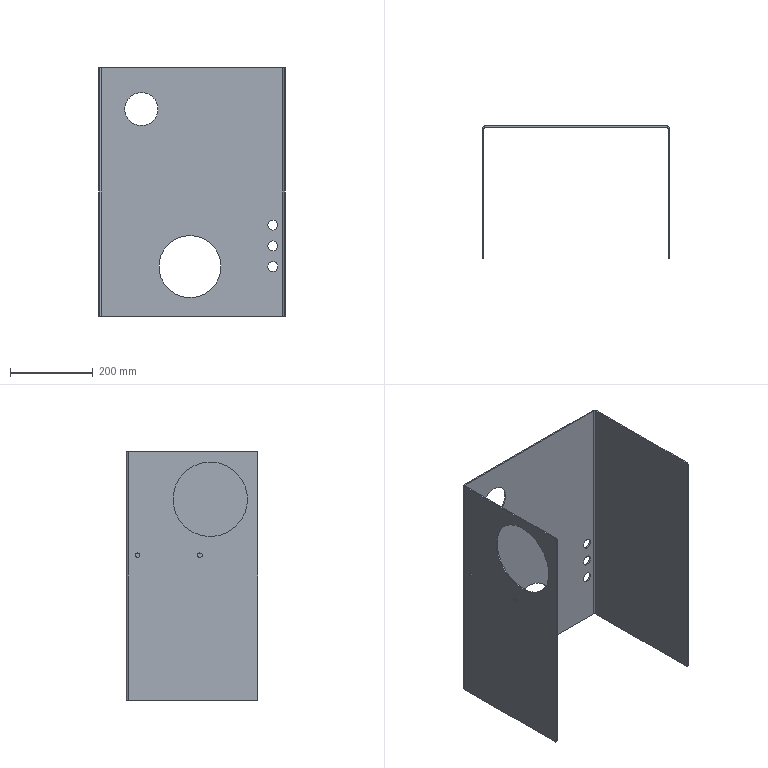Part | SolidWorks | features ICE 3, FlatPattern 1, SMBaseFlange 1, SheetMetal 1 | 1 solid | 42 faces | box 450 x 318 x 600 mm | volume 1787947 mm3 | cylinder 24 | plane 18 | commonest cylinder face diameters 6 x6 24 x6 11 x4 12 x2 80 x2 150 x2
STEP:
#1=CARTESIAN_POINT('',(3.,140.,344.5));
#2=VERTEX_POINT('',#1);
#3=CARTESIAN_POINT('',(3.,140.,355.5));
#4=VERTEX_POINT('',#3);
#5=CARTESIAN_POINT('',(3.,140.,350.));
#6=DIRECTION('',(-1.,0.,0.));
#7=DIRECTION('',(0.,0.,1.));
#8=AXIS2_PLACEMENT_3D('',#5,#6,#7);
#9=CIRCLE('',#8,5.5);
#10=EDGE_CURVE('',#2,#4,#9,.T.);
#11=ORIENTED_EDGE('',*,*,#10,.F.);
#12=CARTESIAN_POINT('',(0.,140.,344.5));
#13=VERTEX_POINT('',#12);
#14=CARTESIAN_POINT('',(10.,140.,344.5));
#15=DIRECTION('',(-1.,0.,0.));
#16=VECTOR('',#15,1000.);
#17=LINE('',#14,#16);
#18=EDGE_CURVE('',#2,#13,#17,.T.);
#19=ORIENTED_EDGE('',*,*,#18,.T.);
#20=CARTESIAN_POINT('',(0.,140.,355.5));
#21=VERTEX_POINT('',#20);
#22=CARTESIAN_POINT('',(0.,140.,350.));
#23=DIRECTION('',(-1.,0.,0.));
#24=DIRECTION('',(0.,0.,1.));
#25=AXIS2_PLACEMENT_3D('',#22,#23,#24);
#26=CIRCLE('',#25,5.5);
#27=EDGE_CURVE('',#13,#21,#26,.T.);
#28=ORIENTED_EDGE('',*,*,#27,.T.);
#29=CARTESIAN_POINT('',(10.,140.,355.5));
#30=DIRECTION('',(-1.,0.,0.));
#31=VECTOR('',#30,1000.);
#32=LINE('',#29,#31);
#33=EDGE_CURVE('',#4,#21,#32,.T.);
#34=ORIENTED_EDGE('',*,*,#33,.F.);
#35=EDGE_LOOP('',(#11,#19,#28,#34));
#36=FACE_OUTER_BOUND('',#35,.T.);
#37=CARTESIAN_POINT('',(10.,140.,350.));
#38=DIRECTION('',(-1.,0.,0.));
#39=DIRECTION('',(0.,0.,1.));
#40=AXIS2_PLACEMENT_3D('',#37,#38,#39);
#41=CYLINDRICAL_SURFACE('',#40,5.5);
#42=ADVANCED_FACE('',(#36),#41,.F.);
#43=CARTESIAN_POINT('',(3.,290.,344.5));
#44=VERTEX_POINT('',#43);
#45=CARTESIAN_POINT('',(3.,290.,355.5));
#46=VERTEX_POINT('',#45);
#47=CARTESIAN_POINT('',(3.,290.,350.));
#48=DIRECTION('',(-1.,0.,0.));
#49=DIRECTION('',(0.,0.,1.));
#50=AXIS2_PLACEMENT_3D('',#47,#48,#49);
#51=CIRCLE('',#50,5.5);
#52=EDGE_CURVE('',#44,#46,#51,.T.);
#53=ORIENTED_EDGE('',*,*,#52,.F.);
#54=CARTESIAN_POINT('',(0.,290.,344.5));
#55=VERTEX_POINT('',#54);
#56=CARTESIAN_POINT('',(10.,290.,344.5));
#57=DIRECTION('',(-1.,0.,0.));
#58=VECTOR('',#57,1000.);
#59=LINE('',#56,#58);
#60=EDGE_CURVE('',#44,#55,#59,.T.);
#61=ORIENTED_EDGE('',*,*,#60,.T.);
#62=CARTESIAN_POINT('',(0.,290.,355.5));
#63=VERTEX_POINT('',#62);
#64=CARTESIAN_POINT('',(0.,290.,350.));
#65=DIRECTION('',(-1.,0.,0.));
#66=DIRECTION('',(0.,0.,1.));
#67=AXIS2_PLACEMENT_3D('',#64,#65,#66);
#68=CIRCLE('',#67,5.5);
#69=EDGE_CURVE('',#55,#63,#68,.T.);
#70=ORIENTED_EDGE('',*,*,#69,.T.);
#71=CARTESIAN_POINT('',(10.,290.,355.5));
#72=DIRECTION('',(-1.,0.,0.));
#73=VECTOR('',#72,1000.);
#74=LINE('',#71,#73);
#75=EDGE_CURVE('',#46,#63,#74,.T.);
#76=ORIENTED_EDGE('',*,*,#75,.F.);
#77=EDGE_LOOP('',(#53,#61,#70,#76));
#78=FACE_OUTER_BOUND('',#77,.T.);
#79=CARTESIAN_POINT('',(10.,290.,350.));
#80=DIRECTION('',(-1.,0.,0.));
#81=DIRECTION('',(0.,0.,1.));
#82=AXIS2_PLACEMENT_3D('',#79,#80,#81);
#83=CYLINDRICAL_SURFACE('',#82,5.5);
#84=ADVANCED_FACE('',(#78),#83,.F.);
#85=CARTESIAN_POINT('',(3.,115.,395.));
#86=VERTEX_POINT('',#85);
#87=CARTESIAN_POINT('',(3.,115.,575.));
#88=VERTEX_POINT('',#87);
#89=CARTESIAN_POINT('',(3.,115.,485.));
#90=DIRECTION('',(-1.,0.,0.));
#91=DIRECTION('',(0.,0.,1.));
#92=AXIS2_PLACEMENT_3D('',#89,#90,#91);
#93=CIRCLE('',#92,90.);
#94=EDGE_CURVE('',#86,#88,#93,.T.);
#95=ORIENTED_EDGE('',*,*,#94,.F.);
#96=CARTESIAN_POINT('',(0.,115.,395.));
#97=VERTEX_POINT('',#96);
#98=CARTESIAN_POINT('',(10.,115.,395.));
#99=DIRECTION('',(-1.,0.,0.));
#100=VECTOR('',#99,1000.);
#101=LINE('',#98,#100);
#102=EDGE_CURVE('',#86,#97,#101,.T.);
#103=ORIENTED_EDGE('',*,*,#102,.T.);
#104=CARTESIAN_POINT('',(0.,115.,575.));
#105=VERTEX_POINT('',#104);
#106=CARTESIAN_POINT('',(0.,115.,485.));
#107=DIRECTION('',(-1.,0.,0.));
#108=DIRECTION('',(0.,0.,1.));
#109=AXIS2_PLACEMENT_3D('',#106,#107,#108);
#110=CIRCLE('',#109,90.);
#111=EDGE_CURVE('',#97,#105,#110,.T.);
#112=ORIENTED_EDGE('',*,*,#111,.T.);
#113=CARTESIAN_POINT('',(10.,115.,575.));
#114=DIRECTION('',(-1.,0.,0.));
#115=VECTOR('',#114,1000.);
#116=LINE('',#113,#115);
#117=EDGE_CURVE('',#88,#105,#116,.T.);
#118=ORIENTED_EDGE('',*,*,#117,.F.);
#119=EDGE_LOOP('',(#95,#103,#112,#118));
#120=FACE_OUTER_BOUND('',#119,.T.);
#121=CARTESIAN_POINT('',(10.,115.,485.));
#122=DIRECTION('',(-1.,0.,0.));
#123=DIRECTION('',(0.,0.,1.));
#124=AXIS2_PLACEMENT_3D('',#121,#122,#123);
#125=CYLINDRICAL_SURFACE('',#124,90.);
#126=ADVANCED_FACE('',(#120),#125,.F.);
#127=CARTESIAN_POINT('',(103.,315.,460.));
#128=VERTEX_POINT('',#127);
#129=CARTESIAN_POINT('',(103.,315.,540.));
#130=VERTEX_POINT('',#129);
#131=CARTESIAN_POINT('',(103.,315.,500.));
#132=DIRECTION('',(0.,1.,0.));
#133=DIRECTION('',(0.,0.,1.));
#134=AXIS2_PLACEMENT_3D('',#131,#132,#133);
#135=CIRCLE('',#134,40.);
#136=EDGE_CURVE('',#128,#130,#135,.T.);
#137=ORIENTED_EDGE('',*,*,#136,.F.);
#138=CARTESIAN_POINT('',(103.,318.,460.));
#139=VERTEX_POINT('',#138);
#140=CARTESIAN_POINT('',(103.,308.,460.));
#141=DIRECTION('',(0.,1.,0.));
#142=VECTOR('',#141,1000.);
#143=LINE('',#140,#142);
#144=EDGE_CURVE('',#128,#139,#143,.T.);
#145=ORIENTED_EDGE('',*,*,#144,.T.);
#146=CARTESIAN_POINT('',(103.,318.,540.));
#147=VERTEX_POINT('',#146);
#148=CARTESIAN_POINT('',(103.,318.,500.));
#149=DIRECTION('',(0.,1.,0.));
#150=DIRECTION('',(0.,0.,1.));
#151=AXIS2_PLACEMENT_3D('',#148,#149,#150);
#152=CIRCLE('',#151,40.);
#153=EDGE_CURVE('',#139,#147,#152,.T.);
#154=ORIENTED_EDGE('',*,*,#153,.T.);
#155=CARTESIAN_POINT('',(103.,308.,540.));
#156=DIRECTION('',(0.,1.,0.));
#157=VECTOR('',#156,1000.);
#158=LINE('',#155,#157);
#159=EDGE_CURVE('',#130,#147,#158,.T.);
#160=ORIENTED_EDGE('',*,*,#159,.F.);
#161=EDGE_LOOP('',(#137,#145,#154,#160));
#162=FACE_OUTER_BOUND('',#161,.T.);
#163=CARTESIAN_POINT('',(103.,308.,500.));
#164=DIRECTION('',(0.,1.,0.));
#165=DIRECTION('',(0.,0.,1.));
#166=AXIS2_PLACEMENT_3D('',#163,#164,#165);
#167=CYLINDRICAL_SURFACE('',#166,40.);
#168=ADVANCED_FACE('',(#162),#167,.F.);
#169=CARTESIAN_POINT('',(220.,315.,45.));
#170=VERTEX_POINT('',#169);
#171=CARTESIAN_POINT('',(220.,315.,195.));
#172=VERTEX_POINT('',#171);
#173=CARTESIAN_POINT('',(220.,315.,120.));
#174=DIRECTION('',(0.,1.,0.));
#175=DIRECTION('',(0.,0.,1.));
#176=AXIS2_PLACEMENT_3D('',#173,#174,#175);
#177=CIRCLE('',#176,75.);
#178=EDGE_CURVE('',#170,#172,#177,.T.);
#179=ORIENTED_EDGE('',*,*,#178,.F.);
#180=CARTESIAN_POINT('',(220.,318.,45.));
#181=VERTEX_POINT('',#180);
#182=CARTESIAN_POINT('',(220.,308.,45.));
#183=DIRECTION('',(0.,1.,0.));
#184=VECTOR('',#183,1000.);
#185=LINE('',#182,#184);
#186=EDGE_CURVE('',#170,#181,#185,.T.);
#187=ORIENTED_EDGE('',*,*,#186,.T.);
#188=CARTESIAN_POINT('',(220.,318.,195.));
#189=VERTEX_POINT('',#188);
#190=CARTESIAN_POINT('',(220.,318.,120.));
#191=DIRECTION('',(0.,1.,0.));
#192=DIRECTION('',(0.,0.,1.));
#193=AXIS2_PLACEMENT_3D('',#190,#191,#192);
#194=CIRCLE('',#193,75.);
#195=EDGE_CURVE('',#181,#189,#194,.T.);
#196=ORIENTED_EDGE('',*,*,#195,.T.);
#197=CARTESIAN_POINT('',(220.,308.,195.));
#198=DIRECTION('',(0.,1.,0.));
#199=VECTOR('',#198,1000.);
#200=LINE('',#197,#199);
#201=EDGE_CURVE('',#172,#189,#200,.T.);
#202=ORIENTED_EDGE('',*,*,#201,.F.);
#203=EDGE_LOOP('',(#179,#187,#196,#202));
#204=FACE_OUTER_BOUND('',#203,.T.);
#205=CARTESIAN_POINT('',(220.,308.,120.));
#206=DIRECTION('',(0.,1.,0.));
#207=DIRECTION('',(0.,0.,1.));
#208=AXIS2_PLACEMENT_3D('',#205,#206,#207);
#209=CYLINDRICAL_SURFACE('',#208,75.);
#210=ADVANCED_FACE('',(#204),#209,.F.);
#211=CARTESIAN_POINT('',(420.,315.,208.));
#212=VERTEX_POINT('',#211);
#213=CARTESIAN_POINT('',(420.,315.,232.));
#214=VERTEX_POINT('',#213);
#215=CARTESIAN_POINT('',(420.,315.,220.));
#216=DIRECTION('',(0.,1.,0.));
#217=DIRECTION('',(0.,0.,1.));
#218=AXIS2_PLACEMENT_3D('',#215,#216,#217);
#219=CIRCLE('',#218,12.);
#220=EDGE_CURVE('',#212,#214,#219,.T.);
#221=ORIENTED_EDGE('',*,*,#220,.F.);
#222=CARTESIAN_POINT('',(420.,318.,208.));
#223=VERTEX_POINT('',#222);
#224=CARTESIAN_POINT('',(420.,308.,208.));
#225=DIRECTION('',(0.,1.,0.));
#226=VECTOR('',#225,1000.);
#227=LINE('',#224,#226);
#228=EDGE_CURVE('',#212,#223,#227,.T.);
#229=ORIENTED_EDGE('',*,*,#228,.T.);
#230=CARTESIAN_POINT('',(420.,318.,232.));
#231=VERTEX_POINT('',#230);
#232=CARTESIAN_POINT('',(420.,318.,220.));
#233=DIRECTION('',(0.,1.,0.));
#234=DIRECTION('',(0.,0.,1.));
#235=AXIS2_PLACEMENT_3D('',#232,#233,#234);
#236=CIRCLE('',#235,12.);
#237=EDGE_CURVE('',#223,#231,#236,.T.);
#238=ORIENTED_EDGE('',*,*,#237,.T.);
#239=CARTESIAN_POINT('',(420.,308.,232.));
#240=DIRECTION('',(0.,1.,0.));
#241=VECTOR('',#240,1000.);
#242=LINE('',#239,#241);
#243=EDGE_CURVE('',#214,#231,#242,.T.);
#244=ORIENTED_EDGE('',*,*,#243,.F.);
#245=EDGE_LOOP('',(#221,#229,#238,#244));
#246=FACE_OUTER_BOUND('',#245,.T.);
#247=CARTESIAN_POINT('',(420.,308.,220.));
#248=DIRECTION('',(0.,1.,0.));
#249=DIRECTION('',(0.,0.,1.));
#250=AXIS2_PLACEMENT_3D('',#247,#248,#249);
#251=CYLINDRICAL_SURFACE('',#250,12.);
#252=ADVANCED_FACE('',(#246),#251,.F.);
#253=CARTESIAN_POINT('',(420.,315.,158.));
#254=VERTEX_POINT('',#253);
#255=CARTESIAN_POINT('',(420.,315.,182.));
#256=VERTEX_POINT('',#255);
#257=CARTESIAN_POINT('',(420.,315.,170.));
#258=DIRECTION('',(0.,1.,0.));
#259=DIRECTION('',(0.,0.,1.));
#260=AXIS2_PLACEMENT_3D('',#257,#258,#259);
#261=CIRCLE('',#260,12.);
#262=EDGE_CURVE('',#254,#256,#261,.T.);
#263=ORIENTED_EDGE('',*,*,#262,.F.);
#264=CARTESIAN_POINT('',(420.,318.,158.));
#265=VERTEX_POINT('',#264);
#266=CARTESIAN_POINT('',(420.,308.,158.));
#267=DIRECTION('',(0.,1.,0.));
#268=VECTOR('',#267,1000.);
#269=LINE('',#266,#268);
#270=EDGE_CURVE('',#254,#265,#269,.T.);
#271=ORIENTED_EDGE('',*,*,#270,.T.);
#272=CARTESIAN_POINT('',(420.,318.,182.));
#273=VERTEX_POINT('',#272);
#274=CARTESIAN_POINT('',(420.,318.,170.));
#275=DIRECTION('',(0.,1.,0.));
#276=DIRECTION('',(0.,0.,1.));
#277=AXIS2_PLACEMENT_3D('',#274,#275,#276);
#278=CIRCLE('',#277,12.);
#279=EDGE_CURVE('',#265,#273,#278,.T.);
#280=ORIENTED_EDGE('',*,*,#279,.T.);
#281=CARTESIAN_POINT('',(420.,308.,182.));
#282=DIRECTION('',(0.,1.,0.));
#283=VECTOR('',#282,1000.);
#284=LINE('',#281,#283);
#285=EDGE_CURVE('',#256,#273,#284,.T.);
#286=ORIENTED_EDGE('',*,*,#285,.F.);
#287=EDGE_LOOP('',(#263,#271,#280,#286));
#288=FACE_OUTER_BOUND('',#287,.T.);
#289=CARTESIAN_POINT('',(420.,308.,170.));
#290=DIRECTION('',(0.,1.,0.));
#291=DIRECTION('',(0.,0.,1.));
#292=AXIS2_PLACEMENT_3D('',#289,#290,#291);
#293=CYLINDRICAL_SURFACE('',#292,12.);
#294=ADVANCED_FACE('',(#288),#293,.F.);
#295=CARTESIAN_POINT('',(420.,315.,108.));
#296=VERTEX_POINT('',#295);
#297=CARTESIAN_POINT('',(420.,315.,132.));
#298=VERTEX_POINT('',#297);
#299=CARTESIAN_POINT('',(420.,315.,120.));
#300=DIRECTION('',(0.,1.,0.));
#301=DIRECTION('',(0.,0.,1.));
#302=AXIS2_PLACEMENT_3D('',#299,#300,#301);
#303=CIRCLE('',#302,12.);
#304=EDGE_CURVE('',#296,#298,#303,.T.);
#305=ORIENTED_EDGE('',*,*,#304,.F.);
#306=CARTESIAN_POINT('',(420.,318.,108.));
#307=VERTEX_POINT('',#306);
#308=CARTESIAN_POINT('',(420.,308.,108.));
#309=DIRECTION('',(0.,1.,0.));
#310=VECTOR('',#309,1000.);
#311=LINE('',#308,#310);
#312=EDGE_CURVE('',#296,#307,#311,.T.);
#313=ORIENTED_EDGE('',*,*,#312,.T.);
#314=CARTESIAN_POINT('',(420.,318.,132.));
#315=VERTEX_POINT('',#314);
#316=CARTESIAN_POINT('',(420.,318.,120.));
#317=DIRECTION('',(0.,1.,0.));
#318=DIRECTION('',(0.,0.,1.));
#319=AXIS2_PLACEMENT_3D('',#316,#317,#318);
#320=CIRCLE('',#319,12.);
#321=EDGE_CURVE('',#307,#315,#320,.T.);
#322=ORIENTED_EDGE('',*,*,#321,.T.);
#323=CARTESIAN_POINT('',(420.,308.,132.));
#324=DIRECTION('',(0.,1.,0.));
#325=VECTOR('',#324,1000.);
#326=LINE('',#323,#325);
#327=EDGE_CURVE('',#298,#315,#326,.T.);
#328=ORIENTED_EDGE('',*,*,#327,.F.);
#329=EDGE_LOOP('',(#305,#313,#322,#328));
#330=FACE_OUTER_BOUND('',#329,.T.);
#331=CARTESIAN_POINT('',(420.,308.,120.));
#332=DIRECTION('',(0.,1.,0.));
#333=DIRECTION('',(0.,0.,1.));
#334=AXIS2_PLACEMENT_3D('',#331,#332,#333);
#335=CYLINDRICAL_SURFACE('',#334,12.);
#336=ADVANCED_FACE('',(#330),#335,.F.);
#337=CARTESIAN_POINT('',(447.,0.,597.));
#338=VERTEX_POINT('',#337);
#339=CARTESIAN_POINT('',(447.,3.,600.));
#340=VERTEX_POINT('',#339);
#341=CARTESIAN_POINT('',(447.,3.,597.));
#342=DIRECTION('',(-1.,0.,0.));
#343=DIRECTION('',(0.,1.,0.));
#344=AXIS2_PLACEMENT_3D('',#341,#342,#343);
#345=CIRCLE('',#344,3.);
#346=EDGE_CURVE('',#338,#340,#345,.T.);
#347=ORIENTED_EDGE('',*,*,#346,.T.);
#348=CARTESIAN_POINT('',(447.,312.,600.));
#349=VERTEX_POINT('',#348);
#350=CARTESIAN_POINT('',(447.,318.,600.));
#351=DIRECTION('',(0.,-1.,0.));
#352=VECTOR('',#351,1000.);
#353=LINE('',#350,#352);
#354=EDGE_CURVE('',#349,#340,#353,.T.);
#355=ORIENTED_EDGE('',*,*,#354,.F.);
#356=CARTESIAN_POINT('',(447.,312.,0.));
#357=VERTEX_POINT('',#356);
#358=CARTESIAN_POINT('',(447.,312.,600.));
#359=DIRECTION('',(0.,0.,-1.));
#360=VECTOR('',#359,1000.);
#361=LINE('',#358,#360);
#362=EDGE_CURVE('',#349,#357,#361,.T.);
#363=ORIENTED_EDGE('',*,*,#362,.T.);
#364=CARTESIAN_POINT('',(447.,3.,0.));
#365=VERTEX_POINT('',#364);
#366=CARTESIAN_POINT('',(447.,318.,0.));
#367=DIRECTION('',(0.,-1.,0.));
#368=VECTOR('',#367,1000.);
#369=LINE('',#366,#368);
#370=EDGE_CURVE('',#357,#365,#369,.T.);
#371=ORIENTED_EDGE('',*,*,#370,.T.);
#372=CARTESIAN_POINT('',(447.,0.,3.));
#373=VERTEX_POINT('',#372);
#374=CARTESIAN_POINT('',(447.,3.,3.));
#375=DIRECTION('',(-1.,0.,0.));
#376=DIRECTION('',(0.,1.,0.));
#377=AXIS2_PLACEMENT_3D('',#374,#375,#376);
#378=CIRCLE('',#377,3.);
#379=EDGE_CURVE('',#365,#373,#378,.T.);
#380=ORIENTED_EDGE('',*,*,#379,.T.);
#381=CARTESIAN_POINT('',(447.,0.,600.));
#382=DIRECTION('',(0.,0.,-1.));
#383=VECTOR('',#382,1000.);
#384=LINE('',#381,#383);
#385=EDGE_CURVE('',#338,#373,#384,.T.);
#386=ORIENTED_EDGE('',*,*,#385,.F.);
#387=EDGE_LOOP('',(#347,#355,#363,#371,#380,#386));
#388=FACE_OUTER_BOUND('',#387,.T.);
#389=CARTESIAN_POINT('',(447.,318.,600.));
#390=DIRECTION('',(1.,0.,0.));
#391=DIRECTION('',(0.,1.,0.));
#392=AXIS2_PLACEMENT_3D('',#389,#390,#391);
#393=PLANE('',#392);
#394=ADVANCED_FACE('',(#388),#393,.F.);
#395=CARTESIAN_POINT('',(450.,312.,600.));
#396=VERTEX_POINT('',#395);
#397=CARTESIAN_POINT('',(450.,3.,600.));
#398=VERTEX_POINT('',#397);
#399=CARTESIAN_POINT('',(450.,318.,600.));
#400=DIRECTION('',(0.,-1.,0.));
#401=VECTOR('',#400,1000.);
#402=LINE('',#399,#401);
#403=EDGE_CURVE('',#396,#398,#402,.T.);
#404=ORIENTED_EDGE('',*,*,#403,.T.);
#405=CARTESIAN_POINT('',(450.,0.,597.));
#406=VERTEX_POINT('',#405);
#407=CARTESIAN_POINT('',(450.,3.,597.));
#408=DIRECTION('',(-1.,0.,0.));
#409=DIRECTION('',(0.,1.,0.));
#410=AXIS2_PLACEMENT_3D('',#407,#408,#409);
#411=CIRCLE('',#410,3.);
#412=EDGE_CURVE('',#406,#398,#411,.T.);
#413=ORIENTED_EDGE('',*,*,#412,.F.);
#414=CARTESIAN_POINT('',(450.,0.,3.));
#415=VERTEX_POINT('',#414);
#416=CARTESIAN_POINT('',(450.,0.,600.));
#417=DIRECTION('',(0.,0.,-1.));
#418=VECTOR('',#417,1000.);
#419=LINE('',#416,#418);
#420=EDGE_CURVE('',#406,#415,#419,.T.);
#421=ORIENTED_EDGE('',*,*,#420,.T.);
#422=CARTESIAN_POINT('',(450.,3.,0.));
#423=VERTEX_POINT('',#422);
#424=CARTESIAN_POINT('',(450.,3.,3.));
#425=DIRECTION('',(-1.,0.,0.));
#426=DIRECTION('',(0.,1.,0.));
#427=AXIS2_PLACEMENT_3D('',#424,#425,#426);
#428=CIRCLE('',#427,3.);
#429=EDGE_CURVE('',#423,#415,#428,.T.);
#430=ORIENTED_EDGE('',*,*,#429,.F.);
#431=CARTESIAN_POINT('',(450.,312.,0.));
#432=VERTEX_POINT('',#431);
#433=CARTESIAN_POINT('',(450.,318.,0.));
#434=DIRECTION('',(0.,-1.,0.));
#435=VECTOR('',#434,1000.);
#436=LINE('',#433,#435);
#437=EDGE_CURVE('',#432,#423,#436,.T.);
#438=ORIENTED_EDGE('',*,*,#437,.F.);
#439=CARTESIAN_POINT('',(450.,312.,600.));
#440=DIRECTION('',(0.,0.,-1.));
#441=VECTOR('',#440,1000.);
#442=LINE('',#439,#441);
#443=EDGE_CURVE('',#396,#432,#442,.T.);
#444=ORIENTED_EDGE('',*,*,#443,.F.);
#445=EDGE_LOOP('',(#404,#413,#421,#430,#438,#444));
#446=FACE_OUTER_BOUND('',#445,.T.);
#447=CARTESIAN_POINT('',(450.,318.,600.));
#448=DIRECTION('',(1.,0.,0.));
#449=DIRECTION('',(0.,1.,0.));
#450=AXIS2_PLACEMENT_3D('',#447,#448,#449);
#451=PLANE('',#450);
#452=ADVANCED_FACE('',(#446),#451,.T.);
#453=ORIENTED_EDGE('',*,*,#354,.T.);
#454=CARTESIAN_POINT('',(447.,3.,600.));
#455=DIRECTION('',(1.,0.,0.));
#456=VECTOR('',#455,1000.);
#457=LINE('',#454,#456);
#458=EDGE_CURVE('',#340,#398,#457,.T.);
#459=ORIENTED_EDGE('',*,*,#458,.T.);
#460=ORIENTED_EDGE('',*,*,#403,.F.);
#461=CARTESIAN_POINT('',(450.,312.,600.));
#462=DIRECTION('',(-1.,0.,0.));
#463=VECTOR('',#462,1000.);
#464=LINE('',#461,#463);
#465=EDGE_CURVE('',#396,#349,#464,.T.);
#466=ORIENTED_EDGE('',*,*,#465,.T.);
#467=EDGE_LOOP('',(#453,#459,#460,#466));
#468=FACE_OUTER_BOUND('',#467,.T.);
#469=CARTESIAN_POINT('',(444.,315.,600.));
#470=DIRECTION('',(0.,0.,1.));
#471=DIRECTION('',(1.,0.,0.));
#472=AXIS2_PLACEMENT_3D('',#469,#470,#471);
#473=PLANE('',#472);
#474=ADVANCED_FACE('',(#468),#473,.T.);
#475=CARTESIAN_POINT('',(447.,0.,597.));
#476=DIRECTION('',(1.,0.,0.));
#477=VECTOR('',#476,1000.);
#478=LINE('',#475,#477);
#479=EDGE_CURVE('',#338,#406,#478,.T.);
#480=ORIENTED_EDGE('',*,*,#479,.F.);
#481=ORIENTED_EDGE('',*,*,#385,.T.);
#482=CARTESIAN_POINT('',(447.,0.,3.));
#483=DIRECTION('',(1.,0.,0.));
#484=VECTOR('',#483,1000.);
#485=LINE('',#482,#484);
#486=EDGE_CURVE('',#373,#415,#485,.T.);
#487=ORIENTED_EDGE('',*,*,#486,.T.);
#488=ORIENTED_EDGE('',*,*,#420,.F.);
#489=EDGE_LOOP('',(#480,#481,#487,#488));
#490=FACE_OUTER_BOUND('',#489,.T.);
#491=CARTESIAN_POINT('',(450.,0.,600.));
#492=DIRECTION('',(0.,-1.,0.));
#493=DIRECTION('',(0.,0.,-1.));
#494=AXIS2_PLACEMENT_3D('',#491,#492,#493);
#495=PLANE('',#494);
#496=ADVANCED_FACE('',(#490),#495,.T.);
#497=CARTESIAN_POINT('',(447.,3.,0.));
#498=DIRECTION('',(1.,0.,0.));
#499=VECTOR('',#498,1000.);
#500=LINE('',#497,#499);
#501=EDGE_CURVE('',#365,#423,#500,.T.);
#502=ORIENTED_EDGE('',*,*,#501,.F.);
#503=ORIENTED_EDGE('',*,*,#370,.F.);
#504=CARTESIAN_POINT('',(447.,312.,0.));
#505=DIRECTION('',(1.,0.,0.));
#506=VECTOR('',#505,1000.);
#507=LINE('',#504,#506);
#508=EDGE_CURVE('',#357,#432,#507,.T.);
#509=ORIENTED_EDGE('',*,*,#508,.T.);
#510=ORIENTED_EDGE('',*,*,#437,.T.);
#511=EDGE_LOOP('',(#502,#503,#509,#510));
#512=FACE_OUTER_BOUND('',#511,.T.);
#513=CARTESIAN_POINT('',(444.,312.,0.));
#514=DIRECTION('',(0.,0.,1.));
#515=DIRECTION('',(1.,0.,0.));
#516=AXIS2_PLACEMENT_3D('',#513,#514,#515);
#517=PLANE('',#516);
#518=ADVANCED_FACE('',(#512),#517,.F.);
#519=CARTESIAN_POINT('',(0.,140.,350.));
#520=DIRECTION('',(-1.,0.,0.));
#521=DIRECTION('',(0.,0.,1.));
#522=AXIS2_PLACEMENT_3D('',#519,#520,#521);
#523=CIRCLE('',#522,5.5);
#524=EDGE_CURVE('',#21,#13,#523,.T.);
#525=ORIENTED_EDGE('',*,*,#524,.F.);
#526=ORIENTED_EDGE('',*,*,#27,.F.);
#527=EDGE_LOOP('',(#525,#526));
#528=FACE_BOUND('',#527,.T.);
#529=CARTESIAN_POINT('',(0.,290.,350.));
#530=DIRECTION('',(-1.,0.,0.));
#531=DIRECTION('',(0.,0.,1.));
#532=AXIS2_PLACEMENT_3D('',#529,#530,#531);
#533=CIRCLE('',#532,5.5);
#534=EDGE_CURVE('',#63,#55,#533,.T.);
#535=ORIENTED_EDGE('',*,*,#534,.F.);
#536=ORIENTED_EDGE('',*,*,#69,.F.);
#537=EDGE_LOOP('',(#535,#536));
#538=FACE_BOUND('',#537,.T.);
#539=CARTESIAN_POINT('',(0.,115.,485.));
#540=DIRECTION('',(-1.,0.,0.));
#541=DIRECTION('',(0.,0.,1.));
#542=AXIS2_PLACEMENT_3D('',#539,#540,#541);
#543=CIRCLE('',#542,90.);
#544=EDGE_CURVE('',#105,#97,#543,.T.);
#545=ORIENTED_EDGE('',*,*,#544,.F.);
#546=ORIENTED_EDGE('',*,*,#111,.F.);
#547=EDGE_LOOP('',(#545,#546));
#548=FACE_BOUND('',#547,.T.);
#549=CARTESIAN_POINT('',(0.,0.,597.));
#550=VERTEX_POINT('',#549);
#551=CARTESIAN_POINT('',(0.,0.,3.));
#552=VERTEX_POINT('',#551);
#553=CARTESIAN_POINT('',(0.,0.,600.));
#554=DIRECTION('',(0.,0.,-1.));
#555=VECTOR('',#554,1000.);
#556=LINE('',#553,#555);
#557=EDGE_CURVE('',#550,#552,#556,.T.);
#558=ORIENTED_EDGE('',*,*,#557,.F.);
#559=CARTESIAN_POINT('',(0.,3.,600.));
#560=VERTEX_POINT('',#559);
#561=CARTESIAN_POINT('',(0.,3.,597.));
#562=DIRECTION('',(1.,0.,0.));
#563=DIRECTION('',(0.,0.,1.));
#564=AXIS2_PLACEMENT_3D('',#561,#562,#563);
#565=CIRCLE('',#564,3.);
#566=EDGE_CURVE('',#560,#550,#565,.T.);
#567=ORIENTED_EDGE('',*,*,#566,.F.);
#568=CARTESIAN_POINT('',(0.,312.,600.));
#569=VERTEX_POINT('',#568);
#570=CARTESIAN_POINT('',(0.,0.,600.));
#571=DIRECTION('',(0.,1.,0.));
#572=VECTOR('',#571,1000.);
#573=LINE('',#570,#572);
#574=EDGE_CURVE('',#560,#569,#573,.T.);
#575=ORIENTED_EDGE('',*,*,#574,.T.);
#576=CARTESIAN_POINT('',(0.,312.,0.));
#577=VERTEX_POINT('',#576);
#578=CARTESIAN_POINT('',(0.,312.,600.));
#579=DIRECTION('',(0.,0.,-1.));
#580=VECTOR('',#579,1000.);
#581=LINE('',#578,#580);
#582=EDGE_CURVE('',#569,#577,#581,.T.);
#583=ORIENTED_EDGE('',*,*,#582,.T.);
#584=CARTESIAN_POINT('',(0.,3.,0.));
#585=VERTEX_POINT('',#584);
#586=CARTESIAN_POINT('',(0.,0.,0.));
#587=DIRECTION('',(0.,1.,0.));
#588=VECTOR('',#587,1000.);
#589=LINE('',#586,#588);
#590=EDGE_CURVE('',#585,#577,#589,.T.);
#591=ORIENTED_EDGE('',*,*,#590,.F.);
#592=CARTESIAN_POINT('',(0.,3.,3.));
#593=DIRECTION('',(1.,0.,0.));
#594=DIRECTION('',(0.,0.,1.));
#595=AXIS2_PLACEMENT_3D('',#592,#593,#594);
#596=CIRCLE('',#595,3.);
#597=EDGE_CURVE('',#552,#585,#596,.T.);
#598=ORIENTED_EDGE('',*,*,#597,.F.);
#599=EDGE_LOOP('',(#558,#567,#575,#583,#591,#598));
#600=FACE_OUTER_BOUND('',#599,.T.);
#601=CARTESIAN_POINT('',(0.,0.,600.));
#602=DIRECTION('',(-1.,0.,0.));
#603=DIRECTION('',(0.,0.,1.));
#604=AXIS2_PLACEMENT_3D('',#601,#602,#603);
#605=PLANE('',#604);
#606=ADVANCED_FACE('',(#528,#538,#548,#600),#605,.T.);
#607=CARTESIAN_POINT('',(3.,140.,350.));
#608=DIRECTION('',(-1.,0.,0.));
#609=DIRECTION('',(0.,0.,1.));
#610=AXIS2_PLACEMENT_3D('',#607,#608,#609);
#611=CIRCLE('',#610,5.5);
#612=EDGE_CURVE('',#4,#2,#611,.T.);
#613=ORIENTED_EDGE('',*,*,#612,.T.);
#614=ORIENTED_EDGE('',*,*,#10,.T.);
#615=EDGE_LOOP('',(#613,#614));
#616=FACE_BOUND('',#615,.T.);
#617=CARTESIAN_POINT('',(3.,290.,350.));
#618=DIRECTION('',(-1.,0.,0.));
#619=DIRECTION('',(0.,0.,1.));
#620=AXIS2_PLACEMENT_3D('',#617,#618,#619);
#621=CIRCLE('',#620,5.5);
#622=EDGE_CURVE('',#46,#44,#621,.T.);
#623=ORIENTED_EDGE('',*,*,#622,.T.);
#624=ORIENTED_EDGE('',*,*,#52,.T.);
#625=EDGE_LOOP('',(#623,#624));
#626=FACE_BOUND('',#625,.T.);
#627=CARTESIAN_POINT('',(3.,115.,485.));
#628=DIRECTION('',(-1.,0.,0.));
#629=DIRECTION('',(0.,0.,1.));
#630=AXIS2_PLACEMENT_3D('',#627,#628,#629);
#631=CIRCLE('',#630,90.);
#632=EDGE_CURVE('',#88,#86,#631,.T.);
#633=ORIENTED_EDGE('',*,*,#632,.T.);
#634=ORIENTED_EDGE('',*,*,#94,.T.);
#635=EDGE_LOOP('',(#633,#634));
#636=FACE_BOUND('',#635,.T.);
#637=CARTESIAN_POINT('',(3.,3.,600.));
#638=VERTEX_POINT('',#637);
#639=CARTESIAN_POINT('',(3.,0.,597.));
#640=VERTEX_POINT('',#639);
#641=CARTESIAN_POINT('',(3.,3.,597.));
#642=DIRECTION('',(1.,0.,0.));
#643=DIRECTION('',(0.,0.,1.));
#644=AXIS2_PLACEMENT_3D('',#641,#642,#643);
#645=CIRCLE('',#644,3.);
#646=EDGE_CURVE('',#638,#640,#645,.T.);
#647=ORIENTED_EDGE('',*,*,#646,.T.);
#648=CARTESIAN_POINT('',(3.,0.,3.));
#649=VERTEX_POINT('',#648);
#650=CARTESIAN_POINT('',(3.,0.,600.));
#651=DIRECTION('',(0.,0.,-1.));
#652=VECTOR('',#651,1000.);
#653=LINE('',#650,#652);
#654=EDGE_CURVE('',#640,#649,#653,.T.);
#655=ORIENTED_EDGE('',*,*,#654,.T.);
#656=CARTESIAN_POINT('',(3.,3.,0.));
#657=VERTEX_POINT('',#656);
#658=CARTESIAN_POINT('',(3.,3.,3.));
#659=DIRECTION('',(1.,0.,0.));
#660=DIRECTION('',(0.,0.,1.));
#661=AXIS2_PLACEMENT_3D('',#658,#659,#660);
#662=CIRCLE('',#661,3.);
#663=EDGE_CURVE('',#649,#657,#662,.T.);
#664=ORIENTED_EDGE('',*,*,#663,.T.);
#665=CARTESIAN_POINT('',(3.,312.,0.));
#666=VERTEX_POINT('',#665);
#667=CARTESIAN_POINT('',(3.,0.,0.));
#668=DIRECTION('',(0.,1.,0.));
#669=VECTOR('',#668,1000.);
#670=LINE('',#667,#669);
#671=EDGE_CURVE('',#657,#666,#670,.T.);
#672=ORIENTED_EDGE('',*,*,#671,.T.);
#673=CARTESIAN_POINT('',(3.,312.,600.));
#674=VERTEX_POINT('',#673);
#675=CARTESIAN_POINT('',(3.,312.,600.));
#676=DIRECTION('',(0.,0.,-1.));
#677=VECTOR('',#676,1000.);
#678=LINE('',#675,#677);
#679=EDGE_CURVE('',#674,#666,#678,.T.);
#680=ORIENTED_EDGE('',*,*,#679,.F.);
#681=CARTESIAN_POINT('',(3.,0.,600.));
#682=DIRECTION('',(0.,1.,0.));
#683=VECTOR('',#682,1000.);
#684=LINE('',#681,#683);
#685=EDGE_CURVE('',#638,#674,#684,.T.);
#686=ORIENTED_EDGE('',*,*,#685,.F.);
#687=EDGE_LOOP('',(#647,#655,#664,#672,#680,#686));
#688=FACE_OUTER_BOUND('',#687,.T.);
#689=CARTESIAN_POINT('',(3.,0.,600.));
#690=DIRECTION('',(-1.,0.,0.));
#691=DIRECTION('',(0.,0.,1.));
#692=AXIS2_PLACEMENT_3D('',#689,#690,#691);
#693=PLANE('',#692);
#694=ADVANCED_FACE('',(#616,#626,#636,#688),#693,.F.);
#695=ORIENTED_EDGE('',*,*,#654,.F.);
#696=CARTESIAN_POINT('',(3.,0.,597.));
#697=DIRECTION('',(-1.,0.,0.));
#698=VECTOR('',#697,1000.);
#699=LINE('',#696,#698);
#700=EDGE_CURVE('',#640,#550,#699,.T.);
#701=ORIENTED_EDGE('',*,*,#700,.T.);
#702=ORIENTED_EDGE('',*,*,#557,.T.);
#703=CARTESIAN_POINT('',(3.,0.,3.));
#704=DIRECTION('',(-1.,0.,0.));
#705=VECTOR('',#704,1000.);
#706=LINE('',#703,#705);
#707=EDGE_CURVE('',#649,#552,#706,.T.);
#708=ORIENTED_EDGE('',*,*,#707,.F.);
#709=EDGE_LOOP('',(#695,#701,#702,#708));
#710=FACE_OUTER_BOUND('',#709,.T.);
#711=CARTESIAN_POINT('',(3.,0.,600.));
#712=DIRECTION('',(0.,-1.,0.));
#713=DIRECTION('',(0.,0.,-1.));
#714=AXIS2_PLACEMENT_3D('',#711,#712,#713);
#715=PLANE('',#714);
#716=ADVANCED_FACE('',(#710),#715,.T.);
#717=ORIENTED_EDGE('',*,*,#671,.F.);
#718=CARTESIAN_POINT('',(3.,3.,0.));
#719=DIRECTION('',(-1.,0.,0.));
#720=VECTOR('',#719,1000.);
#721=LINE('',#718,#720);
#722=EDGE_CURVE('',#657,#585,#721,.T.);
#723=ORIENTED_EDGE('',*,*,#722,.T.);
#724=ORIENTED_EDGE('',*,*,#590,.T.);
#725=CARTESIAN_POINT('',(0.,312.,0.));
#726=DIRECTION('',(1.,0.,0.));
#727=VECTOR('',#726,1000.);
#728=LINE('',#725,#727);
#729=EDGE_CURVE('',#577,#666,#728,.T.);
#730=ORIENTED_EDGE('',*,*,#729,.T.);
#731=EDGE_LOOP('',(#717,#723,#724,#730));
#732=FACE_OUTER_BOUND('',#731,.T.);
#733=CARTESIAN_POINT('',(6.,315.,0.));
#734=DIRECTION('',(0.,0.,-1.));
#735=DIRECTION('',(-1.,0.,0.));
#736=AXIS2_PLACEMENT_3D('',#733,#734,#735);
#737=PLANE('',#736);
#738=ADVANCED_FACE('',(#732),#737,.T.);
#739=CARTESIAN_POINT('',(6.,318.,600.));
#740=VERTEX_POINT('',#739);
#741=CARTESIAN_POINT('',(6.,315.,600.));
#742=VERTEX_POINT('',#741);
#743=CARTESIAN_POINT('',(6.,318.,600.));
#744=DIRECTION('',(0.,-1.,0.));
#745=VECTOR('',#744,1000.);
#746=LINE('',#743,#745);
#747=EDGE_CURVE('',#740,#742,#746,.T.);
#748=ORIENTED_EDGE('',*,*,#747,.F.);
#749=CARTESIAN_POINT('',(6.,312.,600.));
#750=DIRECTION('',(0.,0.,-1.));
#751=DIRECTION('',(1.,0.,0.));
#752=AXIS2_PLACEMENT_3D('',#749,#750,#751);
#753=CIRCLE('',#752,6.);
#754=EDGE_CURVE('',#569,#740,#753,.T.);
#755=ORIENTED_EDGE('',*,*,#754,.F.);
#756=CARTESIAN_POINT('',(3.,312.,600.));
#757=DIRECTION('',(-1.,0.,0.));
#758=VECTOR('',#757,1000.);
#759=LINE('',#756,#758);
#760=EDGE_CURVE('',#674,#569,#759,.T.);
#761=ORIENTED_EDGE('',*,*,#760,.F.);
#762=CARTESIAN_POINT('',(6.,312.,600.));
#763=DIRECTION('',(0.,0.,-1.));
#764=DIRECTION('',(1.,0.,0.));
#765=AXIS2_PLACEMENT_3D('',#762,#763,#764);
#766=CIRCLE('',#765,3.);
#767=EDGE_CURVE('',#674,#742,#766,.T.);
#768=ORIENTED_EDGE('',*,*,#767,.T.);
#769=EDGE_LOOP('',(#748,#755,#761,#768));
#770=FACE_OUTER_BOUND('',#769,.T.);
#771=CARTESIAN_POINT('',(6.,318.,600.));
#772=DIRECTION('',(0.,0.,1.));
#773=DIRECTION('',(1.,0.,0.));
#774=AXIS2_PLACEMENT_3D('',#771,#772,#773);
#775=PLANE('',#774);
#776=ADVANCED_FACE('',(#770),#775,.T.);
#777=CARTESIAN_POINT('',(444.,318.,600.));
#778=VERTEX_POINT('',#777);
#779=CARTESIAN_POINT('',(0.,318.,600.));
#780=DIRECTION('',(1.,0.,0.));
#781=VECTOR('',#780,1000.);
#782=LINE('',#779,#781);
#783=EDGE_CURVE('',#740,#778,#782,.T.);
#784=ORIENTED_EDGE('',*,*,#783,.F.);
#785=ORIENTED_EDGE('',*,*,#747,.T.);
#786=CARTESIAN_POINT('',(444.,315.,600.));
#787=VERTEX_POINT('',#786);
#788=CARTESIAN_POINT('',(0.,315.,600.));
#789=DIRECTION('',(1.,0.,0.));
#790=VECTOR('',#789,1000.);
#791=LINE('',#788,#790);
#792=EDGE_CURVE('',#742,#787,#791,.T.);
#793=ORIENTED_EDGE('',*,*,#792,.T.);
#794=CARTESIAN_POINT('',(444.,315.,600.));
#795=DIRECTION('',(0.,1.,0.));
#796=VECTOR('',#795,1000.);
#797=LINE('',#794,#796);
#798=EDGE_CURVE('',#787,#778,#797,.T.);
#799=ORIENTED_EDGE('',*,*,#798,.T.);
#800=EDGE_LOOP('',(#784,#785,#793,#799));
#801=FACE_OUTER_BOUND('',#800,.T.);
#802=CARTESIAN_POINT('',(3.,312.,600.));
#803=DIRECTION('',(0.,0.,1.));
#804=DIRECTION('',(1.,0.,0.));
#805=AXIS2_PLACEMENT_3D('',#802,#803,#804);
#806=PLANE('',#805);
#807=ADVANCED_FACE('',(#801),#806,.T.);
#808=ORIENTED_EDGE('',*,*,#729,.F.);
#809=CARTESIAN_POINT('',(6.,318.,0.));
#810=VERTEX_POINT('',#809);
#811=CARTESIAN_POINT('',(6.,312.,0.));
#812=DIRECTION('',(0.,0.,-1.));
#813=DIRECTION('',(1.,0.,0.));
#814=AXIS2_PLACEMENT_3D('',#811,#812,#813);
#815=CIRCLE('',#814,6.);
#816=EDGE_CURVE('',#577,#810,#815,.T.);
#817=ORIENTED_EDGE('',*,*,#816,.T.);
#818=CARTESIAN_POINT('',(6.,315.,0.));
#819=VERTEX_POINT('',#818);
#820=CARTESIAN_POINT('',(6.,315.,0.));
#821=DIRECTION('',(0.,1.,0.));
#822=VECTOR('',#821,1000.);
#823=LINE('',#820,#822);
#824=EDGE_CURVE('',#819,#810,#823,.T.);
#825=ORIENTED_EDGE('',*,*,#824,.F.);
#826=CARTESIAN_POINT('',(6.,312.,0.));
#827=DIRECTION('',(0.,0.,-1.));
#828=DIRECTION('',(1.,0.,0.));
#829=AXIS2_PLACEMENT_3D('',#826,#827,#828);
#830=CIRCLE('',#829,3.);
#831=EDGE_CURVE('',#666,#819,#830,.T.);
#832=ORIENTED_EDGE('',*,*,#831,.F.);
#833=EDGE_LOOP('',(#808,#817,#825,#832));
#834=FACE_OUTER_BOUND('',#833,.T.);
#835=CARTESIAN_POINT('',(0.,312.,0.));
#836=DIRECTION('',(0.,0.,-1.));
#837=DIRECTION('',(-1.,0.,0.));
#838=AXIS2_PLACEMENT_3D('',#835,#836,#837);
#839=PLANE('',#838);
#840=ADVANCED_FACE('',(#834),#839,.T.);
#841=ORIENTED_EDGE('',*,*,#465,.F.);
#842=CARTESIAN_POINT('',(444.,312.,600.));
#843=DIRECTION('',(0.,0.,-1.));
#844=DIRECTION('',(1.,0.,0.));
#845=AXIS2_PLACEMENT_3D('',#842,#843,#844);
#846=CIRCLE('',#845,6.);
#847=EDGE_CURVE('',#778,#396,#846,.T.);
#848=ORIENTED_EDGE('',*,*,#847,.F.);
#849=ORIENTED_EDGE('',*,*,#798,.F.);
#850=CARTESIAN_POINT('',(444.,312.,600.));
#851=DIRECTION('',(0.,0.,-1.));
#852=DIRECTION('',(1.,0.,0.));
#853=AXIS2_PLACEMENT_3D('',#850,#851,#852);
#854=CIRCLE('',#853,3.);
#855=EDGE_CURVE('',#787,#349,#854,.T.);
#856=ORIENTED_EDGE('',*,*,#855,.T.);
#857=EDGE_LOOP('',(#841,#848,#849,#856));
#858=FACE_OUTER_BOUND('',#857,.T.);
#859=CARTESIAN_POINT('',(450.,312.,600.));
#860=DIRECTION('',(0.,0.,1.));
#861=DIRECTION('',(1.,0.,0.));
#862=AXIS2_PLACEMENT_3D('',#859,#860,#861);
#863=PLANE('',#862);
#864=ADVANCED_FACE('',(#858),#863,.T.);
#865=CARTESIAN_POINT('',(444.,318.,0.));
#866=VERTEX_POINT('',#865);
#867=CARTESIAN_POINT('',(444.,315.,0.));
#868=VERTEX_POINT('',#867);
#869=CARTESIAN_POINT('',(444.,318.,0.));
#870=DIRECTION('',(0.,-1.,0.));
#871=VECTOR('',#870,1000.);
#872=LINE('',#869,#871);
#873=EDGE_CURVE('',#866,#868,#872,.T.);
#874=ORIENTED_EDGE('',*,*,#873,.F.);
#875=CARTESIAN_POINT('',(444.,312.,0.));
#876=DIRECTION('',(0.,0.,-1.));
#877=DIRECTION('',(1.,0.,0.));
#878=AXIS2_PLACEMENT_3D('',#875,#876,#877);
#879=CIRCLE('',#878,6.);
#880=EDGE_CURVE('',#866,#432,#879,.T.);
#881=ORIENTED_EDGE('',*,*,#880,.T.);
#882=ORIENTED_EDGE('',*,*,#508,.F.);
#883=CARTESIAN_POINT('',(444.,312.,0.));
#884=DIRECTION('',(0.,0.,-1.));
#885=DIRECTION('',(1.,0.,0.));
#886=AXIS2_PLACEMENT_3D('',#883,#884,#885);
#887=CIRCLE('',#886,3.);
#888=EDGE_CURVE('',#868,#357,#887,.T.);
#889=ORIENTED_EDGE('',*,*,#888,.F.);
#890=EDGE_LOOP('',(#874,#881,#882,#889));
#891=FACE_OUTER_BOUND('',#890,.T.);
#892=CARTESIAN_POINT('',(444.,318.,0.));
#893=DIRECTION('',(0.,0.,-1.));
#894=DIRECTION('',(-1.,0.,0.));
#895=AXIS2_PLACEMENT_3D('',#892,#893,#894);
#896=PLANE('',#895);
#897=ADVANCED_FACE('',(#891),#896,.T.);
#898=CARTESIAN_POINT('',(0.,318.,0.));
#899=DIRECTION('',(1.,0.,0.));
#900=VECTOR('',#899,1000.);
#901=LINE('',#898,#900);
#902=EDGE_CURVE('',#810,#866,#901,.T.);
#903=ORIENTED_EDGE('',*,*,#902,.T.);
#904=ORIENTED_EDGE('',*,*,#873,.T.);
#905=CARTESIAN_POINT('',(0.,315.,0.));
#906=DIRECTION('',(1.,0.,0.));
#907=VECTOR('',#906,1000.);
#908=LINE('',#905,#907);
#909=EDGE_CURVE('',#819,#868,#908,.T.);
#910=ORIENTED_EDGE('',*,*,#909,.F.);
#911=ORIENTED_EDGE('',*,*,#824,.T.);
#912=EDGE_LOOP('',(#903,#904,#910,#911));
#913=FACE_OUTER_BOUND('',#912,.T.);
#914=CARTESIAN_POINT('',(447.,312.,0.));
#915=DIRECTION('',(0.,0.,-1.));
#916=DIRECTION('',(-1.,0.,0.));
#917=AXIS2_PLACEMENT_3D('',#914,#915,#916);
#918=PLANE('',#917);
#919=ADVANCED_FACE('',(#913),#918,.T.);
#920=ORIENTED_EDGE('',*,*,#880,.F.);
#921=CARTESIAN_POINT('',(444.,318.,600.));
#922=DIRECTION('',(0.,0.,-1.));
#923=VECTOR('',#922,1000.);
#924=LINE('',#921,#923);
#925=EDGE_CURVE('',#778,#866,#924,.T.);
#926=ORIENTED_EDGE('',*,*,#925,.F.);
#927=ORIENTED_EDGE('',*,*,#847,.T.);
#928=ORIENTED_EDGE('',*,*,#443,.T.);
#929=EDGE_LOOP('',(#920,#926,#927,#928));
#930=FACE_OUTER_BOUND('',#929,.T.);
#931=CARTESIAN_POINT('',(444.,312.,600.));
#932=DIRECTION('',(0.,0.,-1.));
#933=DIRECTION('',(-1.,0.,0.));
#934=AXIS2_PLACEMENT_3D('',#931,#932,#933);
#935=CYLINDRICAL_SURFACE('',#934,6.);
#936=ADVANCED_FACE('',(#930),#935,.T.);
#937=CARTESIAN_POINT('',(103.,318.,500.));
#938=DIRECTION('',(0.,1.,0.));
#939=DIRECTION('',(0.,0.,1.));
#940=AXIS2_PLACEMENT_3D('',#937,#938,#939);
#941=CIRCLE('',#940,40.);
#942=EDGE_CURVE('',#147,#139,#941,.T.);
#943=ORIENTED_EDGE('',*,*,#942,.F.);
#944=ORIENTED_EDGE('',*,*,#153,.F.);
#945=EDGE_LOOP('',(#943,#944));
#946=FACE_BOUND('',#945,.T.);
#947=CARTESIAN_POINT('',(220.,318.,120.));
#948=DIRECTION('',(0.,1.,0.));
#949=DIRECTION('',(0.,0.,1.));
#950=AXIS2_PLACEMENT_3D('',#947,#948,#949);
#951=CIRCLE('',#950,75.);
#952=EDGE_CURVE('',#189,#181,#951,.T.);
#953=ORIENTED_EDGE('',*,*,#952,.F.);
#954=ORIENTED_EDGE('',*,*,#195,.F.);
#955=EDGE_LOOP('',(#953,#954));
#956=FACE_BOUND('',#955,.T.);
#957=CARTESIAN_POINT('',(420.,318.,220.));
#958=DIRECTION('',(0.,1.,0.));
#959=DIRECTION('',(0.,0.,1.));
#960=AXIS2_PLACEMENT_3D('',#957,#958,#959);
#961=CIRCLE('',#960,12.);
#962=EDGE_CURVE('',#231,#223,#961,.T.);
#963=ORIENTED_EDGE('',*,*,#962,.F.);
#964=ORIENTED_EDGE('',*,*,#237,.F.);
#965=EDGE_LOOP('',(#963,#964));
#966=FACE_BOUND('',#965,.T.);
#967=CARTESIAN_POINT('',(420.,318.,170.));
#968=DIRECTION('',(0.,1.,0.));
#969=DIRECTION('',(0.,0.,1.));
#970=AXIS2_PLACEMENT_3D('',#967,#968,#969);
#971=CIRCLE('',#970,12.);
#972=EDGE_CURVE('',#273,#265,#971,.T.);
#973=ORIENTED_EDGE('',*,*,#972,.F.);
#974=ORIENTED_EDGE('',*,*,#279,.F.);
#975=EDGE_LOOP('',(#973,#974));
#976=FACE_BOUND('',#975,.T.);
#977=CARTESIAN_POINT('',(420.,318.,120.));
#978=DIRECTION('',(0.,1.,0.));
#979=DIRECTION('',(0.,0.,1.));
#980=AXIS2_PLACEMENT_3D('',#977,#978,#979);
#981=CIRCLE('',#980,12.);
#982=EDGE_CURVE('',#315,#307,#981,.T.);
#983=ORIENTED_EDGE('',*,*,#982,.F.);
#984=ORIENTED_EDGE('',*,*,#321,.F.);
#985=EDGE_LOOP('',(#983,#984));
#986=FACE_BOUND('',#985,.T.);
#987=ORIENTED_EDGE('',*,*,#902,.F.);
#988=CARTESIAN_POINT('',(6.,318.,600.));
#989=DIRECTION('',(0.,0.,-1.));
#990=VECTOR('',#989,1000.);
#991=LINE('',#988,#990);
#992=EDGE_CURVE('',#740,#810,#991,.T.);
#993=ORIENTED_EDGE('',*,*,#992,.F.);
#994=ORIENTED_EDGE('',*,*,#783,.T.);
#995=ORIENTED_EDGE('',*,*,#925,.T.);
#996=EDGE_LOOP('',(#987,#993,#994,#995));
#997=FACE_OUTER_BOUND('',#996,.T.);
#998=CARTESIAN_POINT('',(0.,318.,600.));
#999=DIRECTION('',(0.,1.,0.));
#1000=DIRECTION('',(0.,0.,1.));
#1001=AXIS2_PLACEMENT_3D('',#998,#999,#1000);
#1002=PLANE('',#1001);
#1003=ADVANCED_FACE('',(#946,#956,#966,#976,#986,#997),#1002,.T.);
#1004=ORIENTED_EDGE('',*,*,#816,.F.);
#1005=ORIENTED_EDGE('',*,*,#582,.F.);
#1006=ORIENTED_EDGE('',*,*,#754,.T.);
#1007=ORIENTED_EDGE('',*,*,#992,.T.);
#1008=EDGE_LOOP('',(#1004,#1005,#1006,#1007));
#1009=FACE_OUTER_BOUND('',#1008,.T.);
#1010=CARTESIAN_POINT('',(6.,312.,600.));
#1011=DIRECTION('',(0.,0.,-1.));
#1012=DIRECTION('',(-1.,0.,0.));
#1013=AXIS2_PLACEMENT_3D('',#1010,#1011,#1012);
#1014=CYLINDRICAL_SURFACE('',#1013,6.);
#1015=ADVANCED_FACE('',(#1009),#1014,.T.);
#1016=ORIENTED_EDGE('',*,*,#831,.T.);
#1017=CARTESIAN_POINT('',(6.,315.,600.));
#1018=DIRECTION('',(0.,0.,-1.));
#1019=VECTOR('',#1018,1000.);
#1020=LINE('',#1017,#1019);
#1021=EDGE_CURVE('',#742,#819,#1020,.T.);
#1022=ORIENTED_EDGE('',*,*,#1021,.F.);
#1023=ORIENTED_EDGE('',*,*,#767,.F.);
#1024=ORIENTED_EDGE('',*,*,#679,.T.);
#1025=EDGE_LOOP('',(#1016,#1022,#1023,#1024));
#1026=FACE_OUTER_BOUND('',#1025,.T.);
#1027=CARTESIAN_POINT('',(6.,312.,600.));
#1028=DIRECTION('',(0.,0.,-1.));
#1029=DIRECTION('',(-1.,0.,0.));
#1030=AXIS2_PLACEMENT_3D('',#1027,#1028,#1029);
#1031=CYLINDRICAL_SURFACE('',#1030,3.);
#1032=ADVANCED_FACE('',(#1026),#1031,.F.);
#1033=CARTESIAN_POINT('',(103.,315.,500.));
#1034=DIRECTION('',(0.,1.,0.));
#1035=DIRECTION('',(0.,0.,1.));
#1036=AXIS2_PLACEMENT_3D('',#1033,#1034,#1035);
#1037=CIRCLE('',#1036,40.);
#1038=EDGE_CURVE('',#130,#128,#1037,.T.);
#1039=ORIENTED_EDGE('',*,*,#1038,.T.);
#1040=ORIENTED_EDGE('',*,*,#136,.T.);
#1041=EDGE_LOOP('',(#1039,#1040));
#1042=FACE_BOUND('',#1041,.T.);
#1043=CARTESIAN_POINT('',(220.,315.,120.));
#1044=DIRECTION('',(0.,1.,0.));
#1045=DIRECTION('',(0.,0.,1.));
#1046=AXIS2_PLACEMENT_3D('',#1043,#1044,#1045);
#1047=CIRCLE('',#1046,75.);
#1048=EDGE_CURVE('',#172,#170,#1047,.T.);
#1049=ORIENTED_EDGE('',*,*,#1048,.T.);
#1050=ORIENTED_EDGE('',*,*,#178,.T.);
#1051=EDGE_LOOP('',(#1049,#1050));
#1052=FACE_BOUND('',#1051,.T.);
#1053=CARTESIAN_POINT('',(420.,315.,220.));
#1054=DIRECTION('',(0.,1.,0.));
#1055=DIRECTION('',(0.,0.,1.));
#1056=AXIS2_PLACEMENT_3D('',#1053,#1054,#1055);
#1057=CIRCLE('',#1056,12.);
#1058=EDGE_CURVE('',#214,#212,#1057,.T.);
#1059=ORIENTED_EDGE('',*,*,#1058,.T.);
#1060=ORIENTED_EDGE('',*,*,#220,.T.);
#1061=EDGE_LOOP('',(#1059,#1060));
#1062=FACE_BOUND('',#1061,.T.);
#1063=CARTESIAN_POINT('',(420.,315.,170.));
#1064=DIRECTION('',(0.,1.,0.));
#1065=DIRECTION('',(0.,0.,1.));
#1066=AXIS2_PLACEMENT_3D('',#1063,#1064,#1065);
#1067=CIRCLE('',#1066,12.);
#1068=EDGE_CURVE('',#256,#254,#1067,.T.);
#1069=ORIENTED_EDGE('',*,*,#1068,.T.);
#1070=ORIENTED_EDGE('',*,*,#262,.T.);
#1071=EDGE_LOOP('',(#1069,#1070));
#1072=FACE_BOUND('',#1071,.T.);
#1073=CARTESIAN_POINT('',(420.,315.,120.));
#1074=DIRECTION('',(0.,1.,0.));
#1075=DIRECTION('',(0.,0.,1.));
#1076=AXIS2_PLACEMENT_3D('',#1073,#1074,#1075);
#1077=CIRCLE('',#1076,12.);
#1078=EDGE_CURVE('',#298,#296,#1077,.T.);
#1079=ORIENTED_EDGE('',*,*,#1078,.T.);
#1080=ORIENTED_EDGE('',*,*,#304,.T.);
#1081=EDGE_LOOP('',(#1079,#1080));
#1082=FACE_BOUND('',#1081,.T.);
#1083=ORIENTED_EDGE('',*,*,#909,.T.);
#1084=CARTESIAN_POINT('',(444.,315.,600.));
#1085=DIRECTION('',(0.,0.,-1.));
#1086=VECTOR('',#1085,1000.);
#1087=LINE('',#1084,#1086);
#1088=EDGE_CURVE('',#787,#868,#1087,.T.);
#1089=ORIENTED_EDGE('',*,*,#1088,.F.);
#1090=ORIENTED_EDGE('',*,*,#792,.F.);
#1091=ORIENTED_EDGE('',*,*,#1021,.T.);
#1092=EDGE_LOOP('',(#1083,#1089,#1090,#1091));
#1093=FACE_OUTER_BOUND('',#1092,.T.);
#1094=CARTESIAN_POINT('',(0.,315.,600.));
#1095=DIRECTION('',(0.,1.,0.));
#1096=DIRECTION('',(0.,0.,1.));
#1097=AXIS2_PLACEMENT_3D('',#1094,#1095,#1096);
#1098=PLANE('',#1097);
#1099=ADVANCED_FACE('',(#1042,#1052,#1062,#1072,#1082,#1093),#1098,.F.);
#1100=ORIENTED_EDGE('',*,*,#888,.T.);
#1101=ORIENTED_EDGE('',*,*,#362,.F.);
#1102=ORIENTED_EDGE('',*,*,#855,.F.);
#1103=ORIENTED_EDGE('',*,*,#1088,.T.);
#1104=EDGE_LOOP('',(#1100,#1101,#1102,#1103));
#1105=FACE_OUTER_BOUND('',#1104,.T.);
#1106=CARTESIAN_POINT('',(444.,312.,600.));
#1107=DIRECTION('',(0.,0.,-1.));
#1108=DIRECTION('',(-1.,0.,0.));
#1109=AXIS2_PLACEMENT_3D('',#1106,#1107,#1108);
#1110=CYLINDRICAL_SURFACE('',#1109,3.);
#1111=ADVANCED_FACE('',(#1105),#1110,.F.);
#1112=CARTESIAN_POINT('',(3.,3.,600.));
#1113=DIRECTION('',(-1.,0.,0.));
#1114=VECTOR('',#1113,1000.);
#1115=LINE('',#1112,#1114);
#1116=EDGE_CURVE('',#638,#560,#1115,.T.);
#1117=ORIENTED_EDGE('',*,*,#1116,.F.);
#1118=ORIENTED_EDGE('',*,*,#685,.T.);
#1119=ORIENTED_EDGE('',*,*,#760,.T.);
#1120=ORIENTED_EDGE('',*,*,#574,.F.);
#1121=EDGE_LOOP('',(#1117,#1118,#1119,#1120));
#1122=FACE_OUTER_BOUND('',#1121,.T.);
#1123=CARTESIAN_POINT('',(444.,312.,600.));
#1124=DIRECTION('',(0.,0.,1.));
#1125=DIRECTION('',(1.,0.,0.));
#1126=AXIS2_PLACEMENT_3D('',#1123,#1124,#1125);
#1127=PLANE('',#1126);
#1128=ADVANCED_FACE('',(#1122),#1127,.T.);
#1129=ORIENTED_EDGE('',*,*,#312,.F.);
#1130=ORIENTED_EDGE('',*,*,#1078,.F.);
#1131=ORIENTED_EDGE('',*,*,#327,.T.);
#1132=ORIENTED_EDGE('',*,*,#982,.T.);
#1133=EDGE_LOOP('',(#1129,#1130,#1131,#1132));
#1134=FACE_OUTER_BOUND('',#1133,.T.);
#1135=CARTESIAN_POINT('',(420.,308.,120.));
#1136=DIRECTION('',(0.,1.,0.));
#1137=DIRECTION('',(0.,0.,1.));
#1138=AXIS2_PLACEMENT_3D('',#1135,#1136,#1137);
#1139=CYLINDRICAL_SURFACE('',#1138,12.);
#1140=ADVANCED_FACE('',(#1134),#1139,.F.);
#1141=ORIENTED_EDGE('',*,*,#270,.F.);
#1142=ORIENTED_EDGE('',*,*,#1068,.F.);
#1143=ORIENTED_EDGE('',*,*,#285,.T.);
#1144=ORIENTED_EDGE('',*,*,#972,.T.);
#1145=EDGE_LOOP('',(#1141,#1142,#1143,#1144));
#1146=FACE_OUTER_BOUND('',#1145,.T.);
#1147=CARTESIAN_POINT('',(420.,308.,170.));
#1148=DIRECTION('',(0.,1.,0.));
#1149=DIRECTION('',(0.,0.,1.));
#1150=AXIS2_PLACEMENT_3D('',#1147,#1148,#1149);
#1151=CYLINDRICAL_SURFACE('',#1150,12.);
#1152=ADVANCED_FACE('',(#1146),#1151,.F.);
#1153=ORIENTED_EDGE('',*,*,#228,.F.);
#1154=ORIENTED_EDGE('',*,*,#1058,.F.);
#1155=ORIENTED_EDGE('',*,*,#243,.T.);
#1156=ORIENTED_EDGE('',*,*,#962,.T.);
#1157=EDGE_LOOP('',(#1153,#1154,#1155,#1156));
#1158=FACE_OUTER_BOUND('',#1157,.T.);
#1159=CARTESIAN_POINT('',(420.,308.,220.));
#1160=DIRECTION('',(0.,1.,0.));
#1161=DIRECTION('',(0.,0.,1.));
#1162=AXIS2_PLACEMENT_3D('',#1159,#1160,#1161);
#1163=CYLINDRICAL_SURFACE('',#1162,12.);
#1164=ADVANCED_FACE('',(#1158),#1163,.F.);
#1165=ORIENTED_EDGE('',*,*,#186,.F.);
#1166=ORIENTED_EDGE('',*,*,#1048,.F.);
#1167=ORIENTED_EDGE('',*,*,#201,.T.);
#1168=ORIENTED_EDGE('',*,*,#952,.T.);
#1169=EDGE_LOOP('',(#1165,#1166,#1167,#1168));
#1170=FACE_OUTER_BOUND('',#1169,.T.);
#1171=CARTESIAN_POINT('',(220.,308.,120.));
#1172=DIRECTION('',(0.,1.,0.));
#1173=DIRECTION('',(0.,0.,1.));
#1174=AXIS2_PLACEMENT_3D('',#1171,#1172,#1173);
#1175=CYLINDRICAL_SURFACE('',#1174,75.);
#1176=ADVANCED_FACE('',(#1170),#1175,.F.);
#1177=ORIENTED_EDGE('',*,*,#144,.F.);
#1178=ORIENTED_EDGE('',*,*,#1038,.F.);
#1179=ORIENTED_EDGE('',*,*,#159,.T.);
#1180=ORIENTED_EDGE('',*,*,#942,.T.);
#1181=EDGE_LOOP('',(#1177,#1178,#1179,#1180));
#1182=FACE_OUTER_BOUND('',#1181,.T.);
#1183=CARTESIAN_POINT('',(103.,308.,500.));
#1184=DIRECTION('',(0.,1.,0.));
#1185=DIRECTION('',(0.,0.,1.));
#1186=AXIS2_PLACEMENT_3D('',#1183,#1184,#1185);
#1187=CYLINDRICAL_SURFACE('',#1186,40.);
#1188=ADVANCED_FACE('',(#1182),#1187,.F.);
#1189=ORIENTED_EDGE('',*,*,#722,.F.);
#1190=ORIENTED_EDGE('',*,*,#663,.F.);
#1191=ORIENTED_EDGE('',*,*,#707,.T.);
#1192=ORIENTED_EDGE('',*,*,#597,.T.);
#1193=EDGE_LOOP('',(#1189,#1190,#1191,#1192));
#1194=FACE_OUTER_BOUND('',#1193,.T.);
#1195=CARTESIAN_POINT('',(3.,3.,3.));
#1196=DIRECTION('',(-1.,0.,0.));
#1197=DIRECTION('',(0.,0.,1.));
#1198=AXIS2_PLACEMENT_3D('',#1195,#1196,#1197);
#1199=CYLINDRICAL_SURFACE('',#1198,3.);
#1200=ADVANCED_FACE('',(#1194),#1199,.T.);
#1201=ORIENTED_EDGE('',*,*,#700,.F.);
#1202=ORIENTED_EDGE('',*,*,#646,.F.);
#1203=ORIENTED_EDGE('',*,*,#1116,.T.);
#1204=ORIENTED_EDGE('',*,*,#566,.T.);
#1205=EDGE_LOOP('',(#1201,#1202,#1203,#1204));
#1206=FACE_OUTER_BOUND('',#1205,.T.);
#1207=CARTESIAN_POINT('',(3.,3.,597.));
#1208=DIRECTION('',(-1.,0.,0.));
#1209=DIRECTION('',(0.,0.,1.));
#1210=AXIS2_PLACEMENT_3D('',#1207,#1208,#1209);
#1211=CYLINDRICAL_SURFACE('',#1210,3.);
#1212=ADVANCED_FACE('',(#1206),#1211,.T.);
#1213=ORIENTED_EDGE('',*,*,#486,.F.);
#1214=ORIENTED_EDGE('',*,*,#379,.F.);
#1215=ORIENTED_EDGE('',*,*,#501,.T.);
#1216=ORIENTED_EDGE('',*,*,#429,.T.);
#1217=EDGE_LOOP('',(#1213,#1214,#1215,#1216));
#1218=FACE_OUTER_BOUND('',#1217,.T.);
#1219=CARTESIAN_POINT('',(447.,3.,3.));
#1220=DIRECTION('',(1.,0.,0.));
#1221=DIRECTION('',(0.,1.,0.));
#1222=AXIS2_PLACEMENT_3D('',#1219,#1220,#1221);
#1223=CYLINDRICAL_SURFACE('',#1222,3.);
#1224=ADVANCED_FACE('',(#1218),#1223,.T.);
#1225=ORIENTED_EDGE('',*,*,#458,.F.);
#1226=ORIENTED_EDGE('',*,*,#346,.F.);
#1227=ORIENTED_EDGE('',*,*,#479,.T.);
#1228=ORIENTED_EDGE('',*,*,#412,.T.);
#1229=EDGE_LOOP('',(#1225,#1226,#1227,#1228));
#1230=FACE_OUTER_BOUND('',#1229,.T.);
#1231=CARTESIAN_POINT('',(447.,3.,597.));
#1232=DIRECTION('',(1.,0.,0.));
#1233=DIRECTION('',(0.,1.,0.));
#1234=AXIS2_PLACEMENT_3D('',#1231,#1232,#1233);
#1235=CYLINDRICAL_SURFACE('',#1234,3.);
#1236=ADVANCED_FACE('',(#1230),#1235,.T.);
#1237=ORIENTED_EDGE('',*,*,#102,.F.);
#1238=ORIENTED_EDGE('',*,*,#632,.F.);
#1239=ORIENTED_EDGE('',*,*,#117,.T.);
#1240=ORIENTED_EDGE('',*,*,#544,.T.);
#1241=EDGE_LOOP('',(#1237,#1238,#1239,#1240));
#1242=FACE_OUTER_BOUND('',#1241,.T.);
#1243=CARTESIAN_POINT('',(10.,115.,485.));
#1244=DIRECTION('',(-1.,0.,0.));
#1245=DIRECTION('',(0.,0.,1.));
#1246=AXIS2_PLACEMENT_3D('',#1243,#1244,#1245);
#1247=CYLINDRICAL_SURFACE('',#1246,90.);
#1248=ADVANCED_FACE('',(#1242),#1247,.F.);
#1249=ORIENTED_EDGE('',*,*,#60,.F.);
#1250=ORIENTED_EDGE('',*,*,#622,.F.);
#1251=ORIENTED_EDGE('',*,*,#75,.T.);
#1252=ORIENTED_EDGE('',*,*,#534,.T.);
#1253=EDGE_LOOP('',(#1249,#1250,#1251,#1252));
#1254=FACE_OUTER_BOUND('',#1253,.T.);
#1255=CARTESIAN_POINT('',(10.,290.,350.));
#1256=DIRECTION('',(-1.,0.,0.));
#1257=DIRECTION('',(0.,0.,1.));
#1258=AXIS2_PLACEMENT_3D('',#1255,#1256,#1257);
#1259=CYLINDRICAL_SURFACE('',#1258,5.5);
#1260=ADVANCED_FACE('',(#1254),#1259,.F.);
#1261=ORIENTED_EDGE('',*,*,#18,.F.);
#1262=ORIENTED_EDGE('',*,*,#612,.F.);
#1263=ORIENTED_EDGE('',*,*,#33,.T.);
#1264=ORIENTED_EDGE('',*,*,#524,.T.);
#1265=EDGE_LOOP('',(#1261,#1262,#1263,#1264));
#1266=FACE_OUTER_BOUND('',#1265,.T.);
#1267=CARTESIAN_POINT('',(10.,140.,350.));
#1268=DIRECTION('',(-1.,0.,0.));
#1269=DIRECTION('',(0.,0.,1.));
#1270=AXIS2_PLACEMENT_3D('',#1267,#1268,#1269);
#1271=CYLINDRICAL_SURFACE('',#1270,5.5);
#1272=ADVANCED_FACE('',(#1266),#1271,.F.);
#1273=CLOSED_SHELL('',(#42,#84,#126,#168,#210,#252,#294,#336,#394,#452,#474,#496,#518,#606,#694,#716,#738,#776,#807,#840,#864,#897,#919,#936,#1003,#1015,#1032,#1099,#1111,#1128,#1140,#1152,#1164,#1176,#1188,#1200,#1212,#1224,#1236,#1248,#1260,#1272));
#1274=MANIFOLD_SOLID_BREP('',#1273);
#1275=CARTESIAN_POINT('',(0.,0.,0.));
#1276=DIRECTION('',(0.,0.,1.));
#1277=DIRECTION('',(1.,0.,0.));
#1278=AXIS2_PLACEMENT_3D('',#1275,#1276,#1277);
#1279=(LENGTH_UNIT()NAMED_UNIT(*)SI_UNIT(.MILLI.,.METRE.));
#1280=UNCERTAINTY_MEASURE_WITH_UNIT(LENGTH_MEASURE(0.00001),#1279,'','');
#1281=(NAMED_UNIT(*)PLANE_ANGLE_UNIT()SI_UNIT($,.RADIAN.));
#1282=(NAMED_UNIT(*)SI_UNIT($,.STERADIAN.)SOLID_ANGLE_UNIT());
#1283=(GEOMETRIC_REPRESENTATION_CONTEXT(3)GLOBAL_UNCERTAINTY_ASSIGNED_CONTEXT((#1280))GLOBAL_UNIT_ASSIGNED_CONTEXT((#1279,#1281,#1282))REPRESENTATION_CONTEXT('',''));
#1284=ADVANCED_BREP_SHAPE_REPRESENTATION('',(#1274,#1278),#1283);